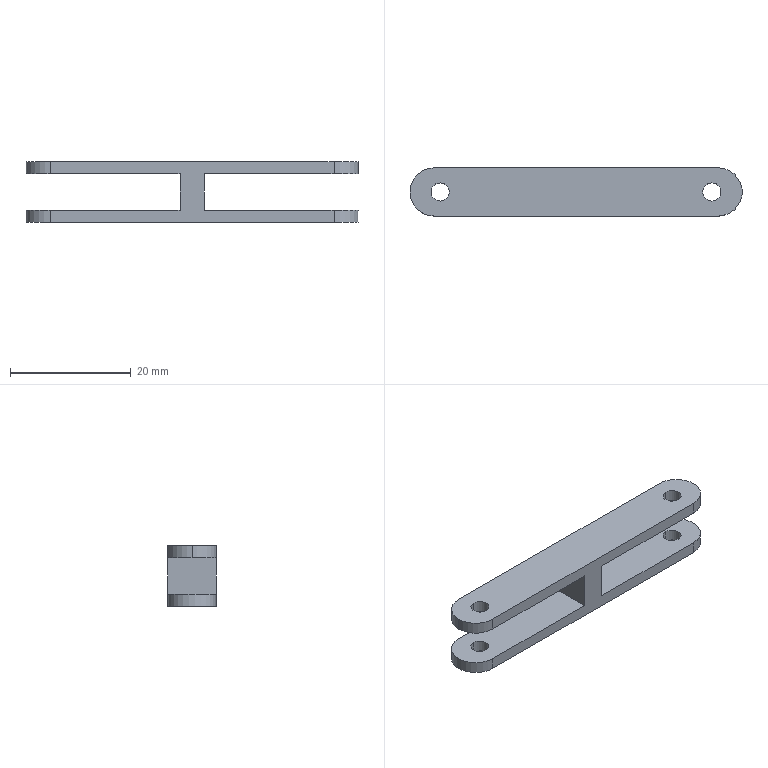Part | SolidWorks | features MBimport 1 | 1 solid | 23 faces | box 55 x 8 x 10 mm | volume 1841 mm3 | cylinder 13 | plane 10 | commonest cylinder face diameters 3 x8 8 x5
STEP:
#1=CARTESIAN_POINT('',(-23.5,4.,8.));
#2=VERTEX_POINT('',#1);
#3=CARTESIAN_POINT('',(-27.5,0.,8.));
#4=VERTEX_POINT('',#3);
#5=CARTESIAN_POINT('',(-23.5,0.,8.));
#6=DIRECTION('',(0.,0.,1.));
#7=DIRECTION('',(0.,1.,0.));
#8=AXIS2_PLACEMENT_3D('',#5,#6,#7);
#9=CIRCLE('',#8,4.);
#10=EDGE_CURVE('',#2,#4,#9,.T.);
#11=ORIENTED_EDGE('',*,*,#10,.T.);
#12=CARTESIAN_POINT('',(-27.5,0.,10.));
#13=VERTEX_POINT('',#12);
#14=CARTESIAN_POINT('',(-27.5,0.,23.036));
#15=DIRECTION('',(0.,0.,1.));
#16=VECTOR('',#15,1000.);
#17=LINE('',#14,#16);
#18=EDGE_CURVE('',#4,#13,#17,.T.);
#19=ORIENTED_EDGE('',*,*,#18,.T.);
#20=CARTESIAN_POINT('',(-23.5,4.,10.));
#21=VERTEX_POINT('',#20);
#22=CARTESIAN_POINT('',(-23.5,0.,10.));
#23=DIRECTION('',(0.,0.,-1.));
#24=DIRECTION('',(0.,-1.,0.));
#25=AXIS2_PLACEMENT_3D('',#22,#23,#24);
#26=CIRCLE('',#25,4.);
#27=EDGE_CURVE('',#13,#21,#26,.T.);
#28=ORIENTED_EDGE('',*,*,#27,.T.);
#29=CARTESIAN_POINT('',(-23.5,4.,10.));
#30=DIRECTION('',(0.,0.,-1.));
#31=VECTOR('',#30,1000.);
#32=LINE('',#29,#31);
#33=EDGE_CURVE('',#21,#2,#32,.T.);
#34=ORIENTED_EDGE('',*,*,#33,.T.);
#35=EDGE_LOOP('',(#11,#19,#28,#34));
#36=FACE_OUTER_BOUND('',#35,.T.);
#37=CARTESIAN_POINT('',(-23.5,0.,23.036));
#38=DIRECTION('',(0.,0.,1.));
#39=DIRECTION('',(-1.,0.,0.));
#40=AXIS2_PLACEMENT_3D('',#37,#38,#39);
#41=CYLINDRICAL_SURFACE('',#40,4.);
#42=ADVANCED_FACE('',(#36),#41,.T.);
#43=CARTESIAN_POINT('',(23.5,4.,0.));
#44=VERTEX_POINT('',#43);
#45=CARTESIAN_POINT('',(-23.5,4.,0.));
#46=VERTEX_POINT('',#45);
#47=CARTESIAN_POINT('',(23.5,4.,0.));
#48=DIRECTION('',(-1.,0.,0.));
#49=VECTOR('',#48,1000.);
#50=LINE('',#47,#49);
#51=EDGE_CURVE('',#44,#46,#50,.T.);
#52=ORIENTED_EDGE('',*,*,#51,.F.);
#53=CARTESIAN_POINT('',(23.5,-4.,0.));
#54=VERTEX_POINT('',#53);
#55=CARTESIAN_POINT('',(23.5,0.,0.));
#56=DIRECTION('',(0.,0.,-1.));
#57=DIRECTION('',(0.,1.,0.));
#58=AXIS2_PLACEMENT_3D('',#55,#56,#57);
#59=CIRCLE('',#58,4.);
#60=EDGE_CURVE('',#44,#54,#59,.T.);
#61=ORIENTED_EDGE('',*,*,#60,.T.);
#62=CARTESIAN_POINT('',(-23.5,-4.,0.));
#63=VERTEX_POINT('',#62);
#64=CARTESIAN_POINT('',(-23.5,-4.,0.));
#65=DIRECTION('',(1.,0.,0.));
#66=VECTOR('',#65,1000.);
#67=LINE('',#64,#66);
#68=EDGE_CURVE('',#63,#54,#67,.T.);
#69=ORIENTED_EDGE('',*,*,#68,.F.);
#70=CARTESIAN_POINT('',(-23.5,0.,0.));
#71=DIRECTION('',(0.,0.,1.));
#72=DIRECTION('',(0.,1.,0.));
#73=AXIS2_PLACEMENT_3D('',#70,#71,#72);
#74=CIRCLE('',#73,4.);
#75=EDGE_CURVE('',#46,#63,#74,.T.);
#76=ORIENTED_EDGE('',*,*,#75,.F.);
#77=EDGE_LOOP('',(#52,#61,#69,#76));
#78=FACE_OUTER_BOUND('',#77,.T.);
#79=CARTESIAN_POINT('',(-22.5,1.5,0.));
#80=VERTEX_POINT('',#79);
#81=CARTESIAN_POINT('',(-22.5,-1.5,0.));
#82=VERTEX_POINT('',#81);
#83=CARTESIAN_POINT('',(-22.5,0.,0.));
#84=DIRECTION('',(0.,0.,1.));
#85=DIRECTION('',(0.,1.,0.));
#86=AXIS2_PLACEMENT_3D('',#83,#84,#85);
#87=CIRCLE('',#86,1.5);
#88=EDGE_CURVE('',#80,#82,#87,.T.);
#89=ORIENTED_EDGE('',*,*,#88,.T.);
#90=CARTESIAN_POINT('',(-22.5,0.,0.));
#91=DIRECTION('',(0.,0.,1.));
#92=DIRECTION('',(0.,-1.,0.));
#93=AXIS2_PLACEMENT_3D('',#90,#91,#92);
#94=CIRCLE('',#93,1.5);
#95=EDGE_CURVE('',#82,#80,#94,.T.);
#96=ORIENTED_EDGE('',*,*,#95,.T.);
#97=EDGE_LOOP('',(#89,#96));
#98=FACE_BOUND('',#97,.T.);
#99=CARTESIAN_POINT('',(22.5,1.5,0.));
#100=VERTEX_POINT('',#99);
#101=CARTESIAN_POINT('',(22.5,-1.5,0.));
#102=VERTEX_POINT('',#101);
#103=CARTESIAN_POINT('',(22.5,0.,0.));
#104=DIRECTION('',(0.,0.,-1.));
#105=DIRECTION('',(0.,1.,0.));
#106=AXIS2_PLACEMENT_3D('',#103,#104,#105);
#107=CIRCLE('',#106,1.5);
#108=EDGE_CURVE('',#100,#102,#107,.T.);
#109=ORIENTED_EDGE('',*,*,#108,.F.);
#110=CARTESIAN_POINT('',(22.5,0.,0.));
#111=DIRECTION('',(0.,0.,-1.));
#112=DIRECTION('',(0.,-1.,0.));
#113=AXIS2_PLACEMENT_3D('',#110,#111,#112);
#114=CIRCLE('',#113,1.5);
#115=EDGE_CURVE('',#102,#100,#114,.T.);
#116=ORIENTED_EDGE('',*,*,#115,.F.);
#117=EDGE_LOOP('',(#109,#116));
#118=FACE_BOUND('',#117,.T.);
#119=CARTESIAN_POINT('',(0.,0.,0.));
#120=DIRECTION('',(0.,0.,1.));
#121=DIRECTION('',(0.,-1.,0.));
#122=AXIS2_PLACEMENT_3D('',#119,#120,#121);
#123=PLANE('',#122);
#124=ADVANCED_FACE('',(#78,#98,#118),#123,.F.);
#125=CARTESIAN_POINT('',(23.5,4.,10.));
#126=VERTEX_POINT('',#125);
#127=CARTESIAN_POINT('',(23.5,4.,10.));
#128=DIRECTION('',(-1.,0.,0.));
#129=VECTOR('',#128,1000.);
#130=LINE('',#127,#129);
#131=EDGE_CURVE('',#126,#21,#130,.T.);
#132=ORIENTED_EDGE('',*,*,#131,.F.);
#133=CARTESIAN_POINT('',(23.5,4.,8.));
#134=VERTEX_POINT('',#133);
#135=CARTESIAN_POINT('',(23.5,4.,10.));
#136=DIRECTION('',(0.,0.,-1.));
#137=VECTOR('',#136,1000.);
#138=LINE('',#135,#137);
#139=EDGE_CURVE('',#126,#134,#138,.T.);
#140=ORIENTED_EDGE('',*,*,#139,.T.);
#141=CARTESIAN_POINT('',(2.,4.,8.));
#142=VERTEX_POINT('',#141);
#143=CARTESIAN_POINT('',(23.5,4.,8.));
#144=DIRECTION('',(-1.,0.,0.));
#145=VECTOR('',#144,1000.);
#146=LINE('',#143,#145);
#147=EDGE_CURVE('',#134,#142,#146,.T.);
#148=ORIENTED_EDGE('',*,*,#147,.T.);
#149=CARTESIAN_POINT('',(2.,4.,2.));
#150=VERTEX_POINT('',#149);
#151=CARTESIAN_POINT('',(2.,4.,2.));
#152=DIRECTION('',(0.,0.,1.));
#153=VECTOR('',#152,1000.);
#154=LINE('',#151,#153);
#155=EDGE_CURVE('',#150,#142,#154,.T.);
#156=ORIENTED_EDGE('',*,*,#155,.F.);
#157=CARTESIAN_POINT('',(23.5,4.,2.));
#158=VERTEX_POINT('',#157);
#159=CARTESIAN_POINT('',(23.5,4.,2.));
#160=DIRECTION('',(-1.,0.,0.));
#161=VECTOR('',#160,1000.);
#162=LINE('',#159,#161);
#163=EDGE_CURVE('',#158,#150,#162,.T.);
#164=ORIENTED_EDGE('',*,*,#163,.F.);
#165=CARTESIAN_POINT('',(23.5,4.,2.));
#166=DIRECTION('',(0.,0.,-1.));
#167=VECTOR('',#166,1000.);
#168=LINE('',#165,#167);
#169=EDGE_CURVE('',#158,#44,#168,.T.);
#170=ORIENTED_EDGE('',*,*,#169,.T.);
#171=ORIENTED_EDGE('',*,*,#51,.T.);
#172=CARTESIAN_POINT('',(-23.5,4.,2.));
#173=VERTEX_POINT('',#172);
#174=CARTESIAN_POINT('',(-23.5,4.,2.));
#175=DIRECTION('',(0.,0.,-1.));
#176=VECTOR('',#175,1000.);
#177=LINE('',#174,#176);
#178=EDGE_CURVE('',#173,#46,#177,.T.);
#179=ORIENTED_EDGE('',*,*,#178,.F.);
#180=CARTESIAN_POINT('',(-2.,4.,2.));
#181=VERTEX_POINT('',#180);
#182=CARTESIAN_POINT('',(-23.5,4.,2.));
#183=DIRECTION('',(1.,0.,0.));
#184=VECTOR('',#183,1000.);
#185=LINE('',#182,#184);
#186=EDGE_CURVE('',#173,#181,#185,.T.);
#187=ORIENTED_EDGE('',*,*,#186,.T.);
#188=CARTESIAN_POINT('',(-2.,4.,8.));
#189=VERTEX_POINT('',#188);
#190=CARTESIAN_POINT('',(-2.,4.,2.));
#191=DIRECTION('',(0.,0.,1.));
#192=VECTOR('',#191,1000.);
#193=LINE('',#190,#192);
#194=EDGE_CURVE('',#181,#189,#193,.T.);
#195=ORIENTED_EDGE('',*,*,#194,.T.);
#196=CARTESIAN_POINT('',(-23.5,4.,8.));
#197=DIRECTION('',(1.,0.,0.));
#198=VECTOR('',#197,1000.);
#199=LINE('',#196,#198);
#200=EDGE_CURVE('',#2,#189,#199,.T.);
#201=ORIENTED_EDGE('',*,*,#200,.F.);
#202=ORIENTED_EDGE('',*,*,#33,.F.);
#203=EDGE_LOOP('',(#132,#140,#148,#156,#164,#170,#171,#179,#187,#195,#201,#202));
#204=FACE_OUTER_BOUND('',#203,.T.);
#205=CARTESIAN_POINT('',(27.5,4.,0.));
#206=DIRECTION('',(0.,1.,0.));
#207=DIRECTION('',(-1.,0.,0.));
#208=AXIS2_PLACEMENT_3D('',#205,#206,#207);
#209=PLANE('',#208);
#210=ADVANCED_FACE('',(#204),#209,.T.);
#211=ORIENTED_EDGE('',*,*,#169,.F.);
#212=CARTESIAN_POINT('',(23.5,-4.,2.));
#213=VERTEX_POINT('',#212);
#214=CARTESIAN_POINT('',(23.5,0.,2.));
#215=DIRECTION('',(0.,0.,1.));
#216=DIRECTION('',(0.,-1.,0.));
#217=AXIS2_PLACEMENT_3D('',#214,#215,#216);
#218=CIRCLE('',#217,4.);
#219=EDGE_CURVE('',#213,#158,#218,.T.);
#220=ORIENTED_EDGE('',*,*,#219,.F.);
#221=CARTESIAN_POINT('',(23.5,-4.,2.));
#222=DIRECTION('',(0.,0.,-1.));
#223=VECTOR('',#222,1000.);
#224=LINE('',#221,#223);
#225=EDGE_CURVE('',#213,#54,#224,.T.);
#226=ORIENTED_EDGE('',*,*,#225,.T.);
#227=ORIENTED_EDGE('',*,*,#60,.F.);
#228=EDGE_LOOP('',(#211,#220,#226,#227));
#229=FACE_OUTER_BOUND('',#228,.T.);
#230=CARTESIAN_POINT('',(23.5,0.,23.036));
#231=DIRECTION('',(0.,0.,1.));
#232=DIRECTION('',(0.,1.,0.));
#233=AXIS2_PLACEMENT_3D('',#230,#231,#232);
#234=CYLINDRICAL_SURFACE('',#233,4.);
#235=ADVANCED_FACE('',(#229),#234,.T.);
#236=CARTESIAN_POINT('',(-23.5,-4.,8.));
#237=VERTEX_POINT('',#236);
#238=CARTESIAN_POINT('',(-2.,-4.,8.));
#239=VERTEX_POINT('',#238);
#240=CARTESIAN_POINT('',(-23.5,-4.,8.));
#241=DIRECTION('',(1.,0.,0.));
#242=VECTOR('',#241,1000.);
#243=LINE('',#240,#242);
#244=EDGE_CURVE('',#237,#239,#243,.T.);
#245=ORIENTED_EDGE('',*,*,#244,.T.);
#246=CARTESIAN_POINT('',(-2.,-4.,2.));
#247=VERTEX_POINT('',#246);
#248=CARTESIAN_POINT('',(-2.,-4.,2.));
#249=DIRECTION('',(0.,0.,1.));
#250=VECTOR('',#249,1000.);
#251=LINE('',#248,#250);
#252=EDGE_CURVE('',#247,#239,#251,.T.);
#253=ORIENTED_EDGE('',*,*,#252,.F.);
#254=CARTESIAN_POINT('',(-23.5,-4.,2.));
#255=VERTEX_POINT('',#254);
#256=CARTESIAN_POINT('',(-23.5,-4.,2.));
#257=DIRECTION('',(1.,0.,0.));
#258=VECTOR('',#257,1000.);
#259=LINE('',#256,#258);
#260=EDGE_CURVE('',#255,#247,#259,.T.);
#261=ORIENTED_EDGE('',*,*,#260,.F.);
#262=CARTESIAN_POINT('',(-23.5,-4.,2.));
#263=DIRECTION('',(0.,0.,-1.));
#264=VECTOR('',#263,1000.);
#265=LINE('',#262,#264);
#266=EDGE_CURVE('',#255,#63,#265,.T.);
#267=ORIENTED_EDGE('',*,*,#266,.T.);
#268=ORIENTED_EDGE('',*,*,#68,.T.);
#269=ORIENTED_EDGE('',*,*,#225,.F.);
#270=CARTESIAN_POINT('',(2.,-4.,2.));
#271=VERTEX_POINT('',#270);
#272=CARTESIAN_POINT('',(23.5,-4.,2.));
#273=DIRECTION('',(-1.,0.,0.));
#274=VECTOR('',#273,1000.);
#275=LINE('',#272,#274);
#276=EDGE_CURVE('',#213,#271,#275,.T.);
#277=ORIENTED_EDGE('',*,*,#276,.T.);
#278=CARTESIAN_POINT('',(2.,-4.,8.));
#279=VERTEX_POINT('',#278);
#280=CARTESIAN_POINT('',(2.,-4.,2.));
#281=DIRECTION('',(0.,0.,1.));
#282=VECTOR('',#281,1000.);
#283=LINE('',#280,#282);
#284=EDGE_CURVE('',#271,#279,#283,.T.);
#285=ORIENTED_EDGE('',*,*,#284,.T.);
#286=CARTESIAN_POINT('',(23.5,-4.,8.));
#287=VERTEX_POINT('',#286);
#288=CARTESIAN_POINT('',(23.5,-4.,8.));
#289=DIRECTION('',(-1.,0.,0.));
#290=VECTOR('',#289,1000.);
#291=LINE('',#288,#290);
#292=EDGE_CURVE('',#287,#279,#291,.T.);
#293=ORIENTED_EDGE('',*,*,#292,.F.);
#294=CARTESIAN_POINT('',(23.5,-4.,10.));
#295=VERTEX_POINT('',#294);
#296=CARTESIAN_POINT('',(23.5,-4.,10.));
#297=DIRECTION('',(0.,0.,-1.));
#298=VECTOR('',#297,1000.);
#299=LINE('',#296,#298);
#300=EDGE_CURVE('',#295,#287,#299,.T.);
#301=ORIENTED_EDGE('',*,*,#300,.F.);
#302=CARTESIAN_POINT('',(-23.5,-4.,10.));
#303=VERTEX_POINT('',#302);
#304=CARTESIAN_POINT('',(-23.5,-4.,10.));
#305=DIRECTION('',(1.,0.,0.));
#306=VECTOR('',#305,1000.);
#307=LINE('',#304,#306);
#308=EDGE_CURVE('',#303,#295,#307,.T.);
#309=ORIENTED_EDGE('',*,*,#308,.F.);
#310=CARTESIAN_POINT('',(-23.5,-4.,10.));
#311=DIRECTION('',(0.,0.,-1.));
#312=VECTOR('',#311,1000.);
#313=LINE('',#310,#312);
#314=EDGE_CURVE('',#303,#237,#313,.T.);
#315=ORIENTED_EDGE('',*,*,#314,.T.);
#316=EDGE_LOOP('',(#245,#253,#261,#267,#268,#269,#277,#285,#293,#301,#309,#315));
#317=FACE_OUTER_BOUND('',#316,.T.);
#318=CARTESIAN_POINT('',(-27.5,-4.,0.));
#319=DIRECTION('',(0.,-1.,0.));
#320=DIRECTION('',(1.,0.,0.));
#321=AXIS2_PLACEMENT_3D('',#318,#319,#320);
#322=PLANE('',#321);
#323=ADVANCED_FACE('',(#317),#322,.T.);
#324=ORIENTED_EDGE('',*,*,#266,.F.);
#325=CARTESIAN_POINT('',(-23.5,0.,2.));
#326=DIRECTION('',(0.,0.,-1.));
#327=DIRECTION('',(0.,-1.,0.));
#328=AXIS2_PLACEMENT_3D('',#325,#326,#327);
#329=CIRCLE('',#328,4.);
#330=EDGE_CURVE('',#255,#173,#329,.T.);
#331=ORIENTED_EDGE('',*,*,#330,.T.);
#332=ORIENTED_EDGE('',*,*,#178,.T.);
#333=ORIENTED_EDGE('',*,*,#75,.T.);
#334=EDGE_LOOP('',(#324,#331,#332,#333));
#335=FACE_OUTER_BOUND('',#334,.T.);
#336=CARTESIAN_POINT('',(-23.5,0.,23.036));
#337=DIRECTION('',(0.,0.,1.));
#338=DIRECTION('',(0.,-1.,0.));
#339=AXIS2_PLACEMENT_3D('',#336,#337,#338);
#340=CYLINDRICAL_SURFACE('',#339,4.);
#341=ADVANCED_FACE('',(#335),#340,.T.);
#342=ORIENTED_EDGE('',*,*,#88,.F.);
#343=CARTESIAN_POINT('',(-22.5,1.5,2.));
#344=VERTEX_POINT('',#343);
#345=CARTESIAN_POINT('',(-22.5,1.5,0.));
#346=DIRECTION('',(0.,0.,1.));
#347=VECTOR('',#346,1000.);
#348=LINE('',#345,#347);
#349=EDGE_CURVE('',#80,#344,#348,.T.);
#350=ORIENTED_EDGE('',*,*,#349,.T.);
#351=CARTESIAN_POINT('',(-22.5,-1.5,2.));
#352=VERTEX_POINT('',#351);
#353=CARTESIAN_POINT('',(-22.5,0.,2.));
#354=DIRECTION('',(0.,0.,1.));
#355=DIRECTION('',(0.,1.,0.));
#356=AXIS2_PLACEMENT_3D('',#353,#354,#355);
#357=CIRCLE('',#356,1.5);
#358=EDGE_CURVE('',#344,#352,#357,.T.);
#359=ORIENTED_EDGE('',*,*,#358,.T.);
#360=CARTESIAN_POINT('',(-22.5,-1.5,0.));
#361=DIRECTION('',(0.,0.,1.));
#362=VECTOR('',#361,1000.);
#363=LINE('',#360,#362);
#364=EDGE_CURVE('',#82,#352,#363,.T.);
#365=ORIENTED_EDGE('',*,*,#364,.F.);
#366=EDGE_LOOP('',(#342,#350,#359,#365));
#367=FACE_OUTER_BOUND('',#366,.T.);
#368=CARTESIAN_POINT('',(-22.5,0.,0.));
#369=DIRECTION('',(0.,0.,-1.));
#370=DIRECTION('',(0.,-1.,0.));
#371=AXIS2_PLACEMENT_3D('',#368,#369,#370);
#372=CYLINDRICAL_SURFACE('',#371,1.5);
#373=ADVANCED_FACE('',(#367),#372,.F.);
#374=CARTESIAN_POINT('',(-22.5,0.,2.));
#375=DIRECTION('',(0.,0.,1.));
#376=DIRECTION('',(0.,-1.,0.));
#377=AXIS2_PLACEMENT_3D('',#374,#375,#376);
#378=CIRCLE('',#377,1.5);
#379=EDGE_CURVE('',#352,#344,#378,.T.);
#380=ORIENTED_EDGE('',*,*,#379,.T.);
#381=ORIENTED_EDGE('',*,*,#349,.F.);
#382=ORIENTED_EDGE('',*,*,#95,.F.);
#383=ORIENTED_EDGE('',*,*,#364,.T.);
#384=EDGE_LOOP('',(#380,#381,#382,#383));
#385=FACE_OUTER_BOUND('',#384,.T.);
#386=CARTESIAN_POINT('',(-22.5,0.,0.));
#387=DIRECTION('',(0.,0.,-1.));
#388=DIRECTION('',(0.,-1.,0.));
#389=AXIS2_PLACEMENT_3D('',#386,#387,#388);
#390=CYLINDRICAL_SURFACE('',#389,1.5);
#391=ADVANCED_FACE('',(#385),#390,.F.);
#392=CARTESIAN_POINT('',(22.5,-1.5,2.));
#393=VERTEX_POINT('',#392);
#394=CARTESIAN_POINT('',(22.5,-1.5,0.));
#395=DIRECTION('',(0.,0.,1.));
#396=VECTOR('',#395,1000.);
#397=LINE('',#394,#396);
#398=EDGE_CURVE('',#102,#393,#397,.T.);
#399=ORIENTED_EDGE('',*,*,#398,.T.);
#400=CARTESIAN_POINT('',(22.5,1.5,2.));
#401=VERTEX_POINT('',#400);
#402=CARTESIAN_POINT('',(22.5,0.,2.));
#403=DIRECTION('',(0.,0.,-1.));
#404=DIRECTION('',(0.,1.,0.));
#405=AXIS2_PLACEMENT_3D('',#402,#403,#404);
#406=CIRCLE('',#405,1.5);
#407=EDGE_CURVE('',#401,#393,#406,.T.);
#408=ORIENTED_EDGE('',*,*,#407,.F.);
#409=CARTESIAN_POINT('',(22.5,1.5,0.));
#410=DIRECTION('',(0.,0.,1.));
#411=VECTOR('',#410,1000.);
#412=LINE('',#409,#411);
#413=EDGE_CURVE('',#100,#401,#412,.T.);
#414=ORIENTED_EDGE('',*,*,#413,.F.);
#415=ORIENTED_EDGE('',*,*,#108,.T.);
#416=EDGE_LOOP('',(#399,#408,#414,#415));
#417=FACE_OUTER_BOUND('',#416,.T.);
#418=CARTESIAN_POINT('',(22.5,0.,0.));
#419=DIRECTION('',(0.,0.,1.));
#420=DIRECTION('',(0.,-1.,0.));
#421=AXIS2_PLACEMENT_3D('',#418,#419,#420);
#422=CYLINDRICAL_SURFACE('',#421,1.5);
#423=ADVANCED_FACE('',(#417),#422,.F.);
#424=ORIENTED_EDGE('',*,*,#413,.T.);
#425=CARTESIAN_POINT('',(22.5,0.,2.));
#426=DIRECTION('',(0.,0.,-1.));
#427=DIRECTION('',(0.,-1.,0.));
#428=AXIS2_PLACEMENT_3D('',#425,#426,#427);
#429=CIRCLE('',#428,1.5);
#430=EDGE_CURVE('',#393,#401,#429,.T.);
#431=ORIENTED_EDGE('',*,*,#430,.F.);
#432=ORIENTED_EDGE('',*,*,#398,.F.);
#433=ORIENTED_EDGE('',*,*,#115,.T.);
#434=EDGE_LOOP('',(#424,#431,#432,#433));
#435=FACE_OUTER_BOUND('',#434,.T.);
#436=CARTESIAN_POINT('',(22.5,0.,0.));
#437=DIRECTION('',(0.,0.,1.));
#438=DIRECTION('',(0.,-1.,0.));
#439=AXIS2_PLACEMENT_3D('',#436,#437,#438);
#440=CYLINDRICAL_SURFACE('',#439,1.5);
#441=ADVANCED_FACE('',(#435),#440,.F.);
#442=ORIENTED_EDGE('',*,*,#308,.T.);
#443=CARTESIAN_POINT('',(23.5,0.,10.));
#444=DIRECTION('',(0.,0.,-1.));
#445=DIRECTION('',(0.,1.,0.));
#446=AXIS2_PLACEMENT_3D('',#443,#444,#445);
#447=CIRCLE('',#446,4.);
#448=EDGE_CURVE('',#126,#295,#447,.T.);
#449=ORIENTED_EDGE('',*,*,#448,.F.);
#450=ORIENTED_EDGE('',*,*,#131,.T.);
#451=ORIENTED_EDGE('',*,*,#27,.F.);
#452=CARTESIAN_POINT('',(-23.5,0.,10.));
#453=DIRECTION('',(0.,0.,-1.));
#454=DIRECTION('',(0.,-1.,0.));
#455=AXIS2_PLACEMENT_3D('',#452,#453,#454);
#456=CIRCLE('',#455,4.);
#457=EDGE_CURVE('',#303,#13,#456,.T.);
#458=ORIENTED_EDGE('',*,*,#457,.F.);
#459=EDGE_LOOP('',(#442,#449,#450,#451,#458));
#460=FACE_OUTER_BOUND('',#459,.T.);
#461=CARTESIAN_POINT('',(-22.5,1.5,10.));
#462=VERTEX_POINT('',#461);
#463=CARTESIAN_POINT('',(-22.5,-1.5,10.));
#464=VERTEX_POINT('',#463);
#465=CARTESIAN_POINT('',(-22.5,0.,10.));
#466=DIRECTION('',(0.,0.,1.));
#467=DIRECTION('',(0.,1.,0.));
#468=AXIS2_PLACEMENT_3D('',#465,#466,#467);
#469=CIRCLE('',#468,1.5);
#470=EDGE_CURVE('',#462,#464,#469,.T.);
#471=ORIENTED_EDGE('',*,*,#470,.F.);
#472=CARTESIAN_POINT('',(-22.5,0.,10.));
#473=DIRECTION('',(0.,0.,1.));
#474=DIRECTION('',(0.,-1.,0.));
#475=AXIS2_PLACEMENT_3D('',#472,#473,#474);
#476=CIRCLE('',#475,1.5);
#477=EDGE_CURVE('',#464,#462,#476,.T.);
#478=ORIENTED_EDGE('',*,*,#477,.F.);
#479=EDGE_LOOP('',(#471,#478));
#480=FACE_BOUND('',#479,.T.);
#481=CARTESIAN_POINT('',(22.5,1.5,10.));
#482=VERTEX_POINT('',#481);
#483=CARTESIAN_POINT('',(22.5,-1.5,10.));
#484=VERTEX_POINT('',#483);
#485=CARTESIAN_POINT('',(22.5,0.,10.));
#486=DIRECTION('',(0.,0.,-1.));
#487=DIRECTION('',(0.,1.,0.));
#488=AXIS2_PLACEMENT_3D('',#485,#486,#487);
#489=CIRCLE('',#488,1.5);
#490=EDGE_CURVE('',#482,#484,#489,.T.);
#491=ORIENTED_EDGE('',*,*,#490,.T.);
#492=CARTESIAN_POINT('',(22.5,0.,10.));
#493=DIRECTION('',(0.,0.,-1.));
#494=DIRECTION('',(0.,-1.,0.));
#495=AXIS2_PLACEMENT_3D('',#492,#493,#494);
#496=CIRCLE('',#495,1.5);
#497=EDGE_CURVE('',#484,#482,#496,.T.);
#498=ORIENTED_EDGE('',*,*,#497,.T.);
#499=EDGE_LOOP('',(#491,#498));
#500=FACE_BOUND('',#499,.T.);
#501=CARTESIAN_POINT('',(0.,0.,10.));
#502=DIRECTION('',(0.,0.,1.));
#503=DIRECTION('',(0.,-1.,0.));
#504=AXIS2_PLACEMENT_3D('',#501,#502,#503);
#505=PLANE('',#504);
#506=ADVANCED_FACE('',(#460,#480,#500),#505,.T.);
#507=ORIENTED_EDGE('',*,*,#139,.F.);
#508=ORIENTED_EDGE('',*,*,#448,.T.);
#509=ORIENTED_EDGE('',*,*,#300,.T.);
#510=CARTESIAN_POINT('',(23.5,0.,8.));
#511=DIRECTION('',(0.,0.,1.));
#512=DIRECTION('',(0.,-1.,0.));
#513=AXIS2_PLACEMENT_3D('',#510,#511,#512);
#514=CIRCLE('',#513,4.);
#515=EDGE_CURVE('',#287,#134,#514,.T.);
#516=ORIENTED_EDGE('',*,*,#515,.T.);
#517=EDGE_LOOP('',(#507,#508,#509,#516));
#518=FACE_OUTER_BOUND('',#517,.T.);
#519=CARTESIAN_POINT('',(23.5,0.,23.036));
#520=DIRECTION('',(0.,0.,1.));
#521=DIRECTION('',(0.,1.,0.));
#522=AXIS2_PLACEMENT_3D('',#519,#520,#521);
#523=CYLINDRICAL_SURFACE('',#522,4.);
#524=ADVANCED_FACE('',(#518),#523,.T.);
#525=CARTESIAN_POINT('',(22.5,1.5,8.));
#526=VERTEX_POINT('',#525);
#527=CARTESIAN_POINT('',(22.5,-1.5,8.));
#528=VERTEX_POINT('',#527);
#529=CARTESIAN_POINT('',(22.5,0.,8.));
#530=DIRECTION('',(0.,0.,-1.));
#531=DIRECTION('',(0.,1.,0.));
#532=AXIS2_PLACEMENT_3D('',#529,#530,#531);
#533=CIRCLE('',#532,1.5);
#534=EDGE_CURVE('',#526,#528,#533,.T.);
#535=ORIENTED_EDGE('',*,*,#534,.F.);
#536=CARTESIAN_POINT('',(22.5,0.,8.));
#537=DIRECTION('',(0.,0.,-1.));
#538=DIRECTION('',(0.,-1.,0.));
#539=AXIS2_PLACEMENT_3D('',#536,#537,#538);
#540=CIRCLE('',#539,1.5);
#541=EDGE_CURVE('',#528,#526,#540,.T.);
#542=ORIENTED_EDGE('',*,*,#541,.F.);
#543=EDGE_LOOP('',(#535,#542));
#544=FACE_BOUND('',#543,.T.);
#545=ORIENTED_EDGE('',*,*,#292,.T.);
#546=CARTESIAN_POINT('',(2.,4.,8.));
#547=DIRECTION('',(0.,-1.,0.));
#548=VECTOR('',#547,1000.);
#549=LINE('',#546,#548);
#550=EDGE_CURVE('',#142,#279,#549,.T.);
#551=ORIENTED_EDGE('',*,*,#550,.F.);
#552=ORIENTED_EDGE('',*,*,#147,.F.);
#553=ORIENTED_EDGE('',*,*,#515,.F.);
#554=EDGE_LOOP('',(#545,#551,#552,#553));
#555=FACE_OUTER_BOUND('',#554,.T.);
#556=CARTESIAN_POINT('',(2.,4.,8.));
#557=DIRECTION('',(0.,0.,1.));
#558=DIRECTION('',(1.,0.,0.));
#559=AXIS2_PLACEMENT_3D('',#556,#557,#558);
#560=PLANE('',#559);
#561=ADVANCED_FACE('',(#544,#555),#560,.F.);
#562=ORIENTED_EDGE('',*,*,#550,.T.);
#563=ORIENTED_EDGE('',*,*,#284,.F.);
#564=CARTESIAN_POINT('',(2.,4.,2.));
#565=DIRECTION('',(0.,-1.,0.));
#566=VECTOR('',#565,1000.);
#567=LINE('',#564,#566);
#568=EDGE_CURVE('',#150,#271,#567,.T.);
#569=ORIENTED_EDGE('',*,*,#568,.F.);
#570=ORIENTED_EDGE('',*,*,#155,.T.);
#571=EDGE_LOOP('',(#562,#563,#569,#570));
#572=FACE_OUTER_BOUND('',#571,.T.);
#573=CARTESIAN_POINT('',(2.,4.,2.));
#574=DIRECTION('',(-1.,0.,0.));
#575=DIRECTION('',(0.,0.,1.));
#576=AXIS2_PLACEMENT_3D('',#573,#574,#575);
#577=PLANE('',#576);
#578=ADVANCED_FACE('',(#572),#577,.F.);
#579=ORIENTED_EDGE('',*,*,#407,.T.);
#580=ORIENTED_EDGE('',*,*,#430,.T.);
#581=EDGE_LOOP('',(#579,#580));
#582=FACE_BOUND('',#581,.T.);
#583=ORIENTED_EDGE('',*,*,#163,.T.);
#584=ORIENTED_EDGE('',*,*,#568,.T.);
#585=ORIENTED_EDGE('',*,*,#276,.F.);
#586=ORIENTED_EDGE('',*,*,#219,.T.);
#587=EDGE_LOOP('',(#583,#584,#585,#586));
#588=FACE_OUTER_BOUND('',#587,.T.);
#589=CARTESIAN_POINT('',(52.,4.,2.));
#590=DIRECTION('',(0.,0.,-1.));
#591=DIRECTION('',(-1.,0.,0.));
#592=AXIS2_PLACEMENT_3D('',#589,#590,#591);
#593=PLANE('',#592);
#594=ADVANCED_FACE('',(#582,#588),#593,.F.);
#595=ORIENTED_EDGE('',*,*,#260,.T.);
#596=CARTESIAN_POINT('',(-2.,4.,2.));
#597=DIRECTION('',(0.,-1.,0.));
#598=VECTOR('',#597,1000.);
#599=LINE('',#596,#598);
#600=EDGE_CURVE('',#181,#247,#599,.T.);
#601=ORIENTED_EDGE('',*,*,#600,.F.);
#602=ORIENTED_EDGE('',*,*,#186,.F.);
#603=ORIENTED_EDGE('',*,*,#330,.F.);
#604=EDGE_LOOP('',(#595,#601,#602,#603));
#605=FACE_OUTER_BOUND('',#604,.T.);
#606=ORIENTED_EDGE('',*,*,#358,.F.);
#607=ORIENTED_EDGE('',*,*,#379,.F.);
#608=EDGE_LOOP('',(#606,#607));
#609=FACE_BOUND('',#608,.T.);
#610=CARTESIAN_POINT('',(-52.,4.,2.));
#611=DIRECTION('',(0.,0.,1.));
#612=DIRECTION('',(1.,0.,0.));
#613=AXIS2_PLACEMENT_3D('',#610,#611,#612);
#614=PLANE('',#613);
#615=ADVANCED_FACE('',(#605,#609),#614,.T.);
#616=ORIENTED_EDGE('',*,*,#252,.T.);
#617=CARTESIAN_POINT('',(-2.,4.,8.));
#618=DIRECTION('',(0.,-1.,0.));
#619=VECTOR('',#618,1000.);
#620=LINE('',#617,#619);
#621=EDGE_CURVE('',#189,#239,#620,.T.);
#622=ORIENTED_EDGE('',*,*,#621,.F.);
#623=ORIENTED_EDGE('',*,*,#194,.F.);
#624=ORIENTED_EDGE('',*,*,#600,.T.);
#625=EDGE_LOOP('',(#616,#622,#623,#624));
#626=FACE_OUTER_BOUND('',#625,.T.);
#627=CARTESIAN_POINT('',(-2.,4.,2.));
#628=DIRECTION('',(-1.,0.,0.));
#629=DIRECTION('',(0.,0.,1.));
#630=AXIS2_PLACEMENT_3D('',#627,#628,#629);
#631=PLANE('',#630);
#632=ADVANCED_FACE('',(#626),#631,.T.);
#633=ORIENTED_EDGE('',*,*,#200,.T.);
#634=ORIENTED_EDGE('',*,*,#621,.T.);
#635=ORIENTED_EDGE('',*,*,#244,.F.);
#636=CARTESIAN_POINT('',(-23.5,0.,8.));
#637=DIRECTION('',(0.,0.,1.));
#638=DIRECTION('',(0.,1.,0.));
#639=AXIS2_PLACEMENT_3D('',#636,#637,#638);
#640=CIRCLE('',#639,4.);
#641=EDGE_CURVE('',#4,#237,#640,.T.);
#642=ORIENTED_EDGE('',*,*,#641,.F.);
#643=ORIENTED_EDGE('',*,*,#10,.F.);
#644=EDGE_LOOP('',(#633,#634,#635,#642,#643));
#645=FACE_OUTER_BOUND('',#644,.T.);
#646=CARTESIAN_POINT('',(-22.5,1.5,8.));
#647=VERTEX_POINT('',#646);
#648=CARTESIAN_POINT('',(-22.5,-1.5,8.));
#649=VERTEX_POINT('',#648);
#650=CARTESIAN_POINT('',(-22.5,0.,8.));
#651=DIRECTION('',(0.,0.,1.));
#652=DIRECTION('',(0.,1.,0.));
#653=AXIS2_PLACEMENT_3D('',#650,#651,#652);
#654=CIRCLE('',#653,1.5);
#655=EDGE_CURVE('',#647,#649,#654,.T.);
#656=ORIENTED_EDGE('',*,*,#655,.T.);
#657=CARTESIAN_POINT('',(-22.5,0.,8.));
#658=DIRECTION('',(0.,0.,1.));
#659=DIRECTION('',(0.,-1.,0.));
#660=AXIS2_PLACEMENT_3D('',#657,#658,#659);
#661=CIRCLE('',#660,1.5);
#662=EDGE_CURVE('',#649,#647,#661,.T.);
#663=ORIENTED_EDGE('',*,*,#662,.T.);
#664=EDGE_LOOP('',(#656,#663));
#665=FACE_BOUND('',#664,.T.);
#666=CARTESIAN_POINT('',(-2.,4.,8.));
#667=DIRECTION('',(0.,0.,-1.));
#668=DIRECTION('',(-1.,0.,0.));
#669=AXIS2_PLACEMENT_3D('',#666,#667,#668);
#670=PLANE('',#669);
#671=ADVANCED_FACE('',(#645,#665),#670,.T.);
#672=ORIENTED_EDGE('',*,*,#18,.F.);
#673=ORIENTED_EDGE('',*,*,#641,.T.);
#674=ORIENTED_EDGE('',*,*,#314,.F.);
#675=ORIENTED_EDGE('',*,*,#457,.T.);
#676=EDGE_LOOP('',(#672,#673,#674,#675));
#677=FACE_OUTER_BOUND('',#676,.T.);
#678=CARTESIAN_POINT('',(-23.5,0.,23.036));
#679=DIRECTION('',(0.,0.,1.));
#680=DIRECTION('',(-1.,0.,0.));
#681=AXIS2_PLACEMENT_3D('',#678,#679,#680);
#682=CYLINDRICAL_SURFACE('',#681,4.);
#683=ADVANCED_FACE('',(#677),#682,.T.);
#684=ORIENTED_EDGE('',*,*,#655,.F.);
#685=CARTESIAN_POINT('',(-22.5,1.5,8.));
#686=DIRECTION('',(0.,0.,1.));
#687=VECTOR('',#686,1000.);
#688=LINE('',#685,#687);
#689=EDGE_CURVE('',#647,#462,#688,.T.);
#690=ORIENTED_EDGE('',*,*,#689,.T.);
#691=ORIENTED_EDGE('',*,*,#470,.T.);
#692=CARTESIAN_POINT('',(-22.5,-1.5,8.));
#693=DIRECTION('',(0.,0.,1.));
#694=VECTOR('',#693,1000.);
#695=LINE('',#692,#694);
#696=EDGE_CURVE('',#649,#464,#695,.T.);
#697=ORIENTED_EDGE('',*,*,#696,.F.);
#698=EDGE_LOOP('',(#684,#690,#691,#697));
#699=FACE_OUTER_BOUND('',#698,.T.);
#700=CARTESIAN_POINT('',(-22.5,0.,0.));
#701=DIRECTION('',(0.,0.,-1.));
#702=DIRECTION('',(0.,-1.,0.));
#703=AXIS2_PLACEMENT_3D('',#700,#701,#702);
#704=CYLINDRICAL_SURFACE('',#703,1.5);
#705=ADVANCED_FACE('',(#699),#704,.F.);
#706=ORIENTED_EDGE('',*,*,#477,.T.);
#707=ORIENTED_EDGE('',*,*,#689,.F.);
#708=ORIENTED_EDGE('',*,*,#662,.F.);
#709=ORIENTED_EDGE('',*,*,#696,.T.);
#710=EDGE_LOOP('',(#706,#707,#708,#709));
#711=FACE_OUTER_BOUND('',#710,.T.);
#712=CARTESIAN_POINT('',(-22.5,0.,0.));
#713=DIRECTION('',(0.,0.,-1.));
#714=DIRECTION('',(0.,-1.,0.));
#715=AXIS2_PLACEMENT_3D('',#712,#713,#714);
#716=CYLINDRICAL_SURFACE('',#715,1.5);
#717=ADVANCED_FACE('',(#711),#716,.F.);
#718=CARTESIAN_POINT('',(22.5,1.5,8.));
#719=DIRECTION('',(0.,0.,1.));
#720=VECTOR('',#719,1000.);
#721=LINE('',#718,#720);
#722=EDGE_CURVE('',#526,#482,#721,.T.);
#723=ORIENTED_EDGE('',*,*,#722,.F.);
#724=ORIENTED_EDGE('',*,*,#534,.T.);
#725=CARTESIAN_POINT('',(22.5,-1.5,8.));
#726=DIRECTION('',(0.,0.,1.));
#727=VECTOR('',#726,1000.);
#728=LINE('',#725,#727);
#729=EDGE_CURVE('',#528,#484,#728,.T.);
#730=ORIENTED_EDGE('',*,*,#729,.T.);
#731=ORIENTED_EDGE('',*,*,#490,.F.);
#732=EDGE_LOOP('',(#723,#724,#730,#731));
#733=FACE_OUTER_BOUND('',#732,.T.);
#734=CARTESIAN_POINT('',(22.5,0.,0.));
#735=DIRECTION('',(0.,0.,1.));
#736=DIRECTION('',(0.,-1.,0.));
#737=AXIS2_PLACEMENT_3D('',#734,#735,#736);
#738=CYLINDRICAL_SURFACE('',#737,1.5);
#739=ADVANCED_FACE('',(#733),#738,.F.);
#740=ORIENTED_EDGE('',*,*,#729,.F.);
#741=ORIENTED_EDGE('',*,*,#541,.T.);
#742=ORIENTED_EDGE('',*,*,#722,.T.);
#743=ORIENTED_EDGE('',*,*,#497,.F.);
#744=EDGE_LOOP('',(#740,#741,#742,#743));
#745=FACE_OUTER_BOUND('',#744,.T.);
#746=CARTESIAN_POINT('',(22.5,0.,0.));
#747=DIRECTION('',(0.,0.,1.));
#748=DIRECTION('',(0.,-1.,0.));
#749=AXIS2_PLACEMENT_3D('',#746,#747,#748);
#750=CYLINDRICAL_SURFACE('',#749,1.5);
#751=ADVANCED_FACE('',(#745),#750,.F.);
#752=CLOSED_SHELL('',(#42,#124,#210,#235,#323,#341,#373,#391,#423,#441,#506,#524,#561,#578,#594,#615,#632,#671,#683,#705,#717,#739,#751));
#753=MANIFOLD_SOLID_BREP('',#752);
#754=CARTESIAN_POINT('',(0.,0.,0.));
#755=DIRECTION('',(0.,0.,1.));
#756=DIRECTION('',(1.,0.,0.));
#757=AXIS2_PLACEMENT_3D('',#754,#755,#756);
#758=(LENGTH_UNIT()NAMED_UNIT(*)SI_UNIT(.MILLI.,.METRE.));
#759=UNCERTAINTY_MEASURE_WITH_UNIT(LENGTH_MEASURE(0.00001),#758,'','');
#760=(NAMED_UNIT(*)PLANE_ANGLE_UNIT()SI_UNIT($,.RADIAN.));
#761=(NAMED_UNIT(*)SI_UNIT($,.STERADIAN.)SOLID_ANGLE_UNIT());
#762=(GEOMETRIC_REPRESENTATION_CONTEXT(3)GLOBAL_UNCERTAINTY_ASSIGNED_CONTEXT((#759))GLOBAL_UNIT_ASSIGNED_CONTEXT((#758,#760,#761))REPRESENTATION_CONTEXT('',''));
#763=ADVANCED_BREP_SHAPE_REPRESENTATION('',(#753,#757),#762);